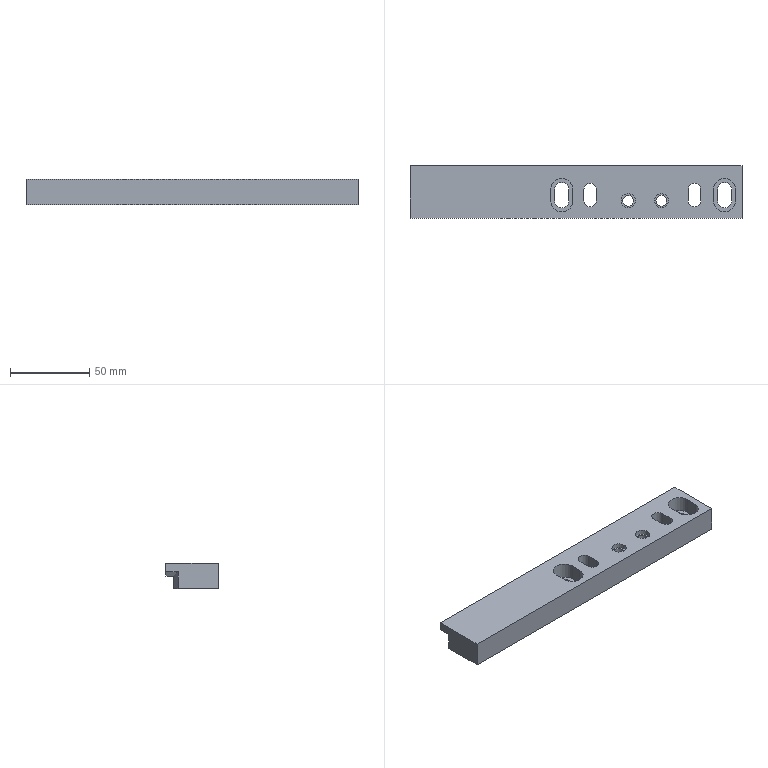Part | STEP file | lll_id4690_x_t | 1 solid | 44 faces | box 210 x 33 x 16 mm | volume 90799 mm3 | plane 28 | cylinder 16 | commonest cylinder face diameters 9 x6 8 x4 14 x4 6.8 x2
STEP:
#1=CARTESIAN_POINT('',(258.835,-359.7,13.));
#2=VERTEX_POINT('',#1);
#3=CARTESIAN_POINT('',(255.435,-359.7,13.));
#4=DIRECTION('',(0.,0.,-1.));
#5=DIRECTION('',(1.,0.,0.));
#6=AXIS2_PLACEMENT_3D('',#3,#4,#5);
#7=CIRCLE('',#6,3.4);
#8=EDGE_CURVE('',#2,#2,#7,.T.);
#9=ORIENTED_EDGE('',*,*,#8,.T.);
#10=EDGE_LOOP('',(#9));
#11=FACE_BOUND('',#10,.T.);
#12=CARTESIAN_POINT('',(250.935,-359.7,13.));
#13=VERTEX_POINT('',#12);
#14=CARTESIAN_POINT('',(255.435,-359.7,13.));
#15=DIRECTION('',(0.,0.,1.));
#16=DIRECTION('',(-1.,0.,0.));
#17=AXIS2_PLACEMENT_3D('',#14,#15,#16);
#18=CIRCLE('',#17,4.5);
#19=EDGE_CURVE('',#13,#13,#18,.T.);
#20=ORIENTED_EDGE('',*,*,#19,.T.);
#21=EDGE_LOOP('',(#20));
#22=FACE_BOUND('',#21,.T.);
#23=CARTESIAN_POINT('',(255.435,-359.7,13.));
#24=DIRECTION('',(0.,0.,-1.));
#25=DIRECTION('',(1.,0.,0.));
#26=AXIS2_PLACEMENT_3D('',#23,#24,#25);
#27=PLANE('',#26);
#28=ADVANCED_FACE('',(#11,#22),#27,.F.);
#29=CARTESIAN_POINT('',(311.935,-359.7,6.));
#30=VERTEX_POINT('',#29);
#31=CARTESIAN_POINT('',(311.935,-352.7,6.));
#32=VERTEX_POINT('',#31);
#33=CARTESIAN_POINT('',(311.935,-352.7,6.));
#34=DIRECTION('',(0.,1.,0.));
#35=VECTOR('',#34,1.);
#36=LINE('',#33,#35);
#37=EDGE_CURVE('',#30,#32,#36,.T.);
#38=ORIENTED_EDGE('',*,*,#37,.T.);
#39=CARTESIAN_POINT('',(320.935,-352.7,6.));
#40=VERTEX_POINT('',#39);
#41=CARTESIAN_POINT('',(316.435,-352.7,6.));
#42=DIRECTION('',(0.,0.,-1.));
#43=DIRECTION('',(1.,0.,0.));
#44=AXIS2_PLACEMENT_3D('',#41,#42,#43);
#45=CIRCLE('',#44,4.5);
#46=EDGE_CURVE('',#32,#40,#45,.T.);
#47=ORIENTED_EDGE('',*,*,#46,.T.);
#48=CARTESIAN_POINT('',(320.935,-359.7,6.));
#49=VERTEX_POINT('',#48);
#50=CARTESIAN_POINT('',(320.935,-359.7,6.));
#51=DIRECTION('',(0.,-1.,0.));
#52=VECTOR('',#51,1.);
#53=LINE('',#50,#52);
#54=EDGE_CURVE('',#40,#49,#53,.T.);
#55=ORIENTED_EDGE('',*,*,#54,.T.);
#56=CARTESIAN_POINT('',(316.435,-359.7,6.));
#57=DIRECTION('',(0.,0.,-1.));
#58=DIRECTION('',(1.,0.,0.));
#59=AXIS2_PLACEMENT_3D('',#56,#57,#58);
#60=CIRCLE('',#59,4.5);
#61=EDGE_CURVE('',#49,#30,#60,.T.);
#62=ORIENTED_EDGE('',*,*,#61,.T.);
#63=EDGE_LOOP('',(#38,#47,#55,#62));
#64=FACE_BOUND('',#63,.T.);
#65=CARTESIAN_POINT('',(323.435,-352.7,6.));
#66=VERTEX_POINT('',#65);
#67=CARTESIAN_POINT('',(309.435,-352.7,6.));
#68=VERTEX_POINT('',#67);
#69=CARTESIAN_POINT('',(316.435,-352.7,6.));
#70=DIRECTION('',(0.,0.,1.));
#71=DIRECTION('',(-1.,0.,0.));
#72=AXIS2_PLACEMENT_3D('',#69,#70,#71);
#73=CIRCLE('',#72,7.);
#74=EDGE_CURVE('',#66,#68,#73,.T.);
#75=ORIENTED_EDGE('',*,*,#74,.T.);
#76=CARTESIAN_POINT('',(309.435,-359.7,6.));
#77=VERTEX_POINT('',#76);
#78=CARTESIAN_POINT('',(309.435,-359.7,6.));
#79=DIRECTION('',(0.,-1.,0.));
#80=VECTOR('',#79,1.);
#81=LINE('',#78,#80);
#82=EDGE_CURVE('',#68,#77,#81,.T.);
#83=ORIENTED_EDGE('',*,*,#82,.T.);
#84=CARTESIAN_POINT('',(323.435,-359.7,6.));
#85=VERTEX_POINT('',#84);
#86=CARTESIAN_POINT('',(316.435,-359.7,6.));
#87=DIRECTION('',(0.,0.,1.));
#88=DIRECTION('',(-1.,0.,0.));
#89=AXIS2_PLACEMENT_3D('',#86,#87,#88);
#90=CIRCLE('',#89,7.);
#91=EDGE_CURVE('',#77,#85,#90,.T.);
#92=ORIENTED_EDGE('',*,*,#91,.T.);
#93=CARTESIAN_POINT('',(323.435,-352.7,6.));
#94=DIRECTION('',(0.,1.,0.));
#95=VECTOR('',#94,1.);
#96=LINE('',#93,#95);
#97=EDGE_CURVE('',#85,#66,#96,.T.);
#98=ORIENTED_EDGE('',*,*,#97,.T.);
#99=EDGE_LOOP('',(#75,#83,#92,#98));
#100=FACE_BOUND('',#99,.T.);
#101=CARTESIAN_POINT('',(316.435,-352.7,6.));
#102=DIRECTION('',(0.,0.,-1.));
#103=DIRECTION('',(1.,0.,0.));
#104=AXIS2_PLACEMENT_3D('',#101,#102,#103);
#105=PLANE('',#104);
#106=ADVANCED_FACE('',(#64,#100),#105,.F.);
#107=CARTESIAN_POINT('',(206.435,-359.7,6.));
#108=VERTEX_POINT('',#107);
#109=CARTESIAN_POINT('',(220.435,-359.7,6.));
#110=VERTEX_POINT('',#109);
#111=CARTESIAN_POINT('',(213.435,-359.7,6.));
#112=DIRECTION('',(0.,0.,1.));
#113=DIRECTION('',(-1.,0.,0.));
#114=AXIS2_PLACEMENT_3D('',#111,#112,#113);
#115=CIRCLE('',#114,7.);
#116=EDGE_CURVE('',#108,#110,#115,.T.);
#117=ORIENTED_EDGE('',*,*,#116,.T.);
#118=CARTESIAN_POINT('',(220.435,-352.7,6.));
#119=VERTEX_POINT('',#118);
#120=CARTESIAN_POINT('',(220.435,-352.7,6.));
#121=DIRECTION('',(0.,1.,0.));
#122=VECTOR('',#121,1.);
#123=LINE('',#120,#122);
#124=EDGE_CURVE('',#110,#119,#123,.T.);
#125=ORIENTED_EDGE('',*,*,#124,.T.);
#126=CARTESIAN_POINT('',(206.435,-352.7,6.));
#127=VERTEX_POINT('',#126);
#128=CARTESIAN_POINT('',(213.435,-352.7,6.));
#129=DIRECTION('',(0.,0.,1.));
#130=DIRECTION('',(-1.,0.,0.));
#131=AXIS2_PLACEMENT_3D('',#128,#129,#130);
#132=CIRCLE('',#131,7.);
#133=EDGE_CURVE('',#119,#127,#132,.T.);
#134=ORIENTED_EDGE('',*,*,#133,.T.);
#135=CARTESIAN_POINT('',(206.435,-359.7,6.));
#136=DIRECTION('',(0.,-1.,0.));
#137=VECTOR('',#136,1.);
#138=LINE('',#135,#137);
#139=EDGE_CURVE('',#127,#108,#138,.T.);
#140=ORIENTED_EDGE('',*,*,#139,.T.);
#141=EDGE_LOOP('',(#117,#125,#134,#140));
#142=FACE_BOUND('',#141,.T.);
#143=CARTESIAN_POINT('',(217.935,-359.7,6.));
#144=VERTEX_POINT('',#143);
#145=CARTESIAN_POINT('',(217.935,-352.7,6.));
#146=VERTEX_POINT('',#145);
#147=CARTESIAN_POINT('',(217.935,-352.7,6.));
#148=DIRECTION('',(0.,1.,0.));
#149=VECTOR('',#148,1.);
#150=LINE('',#147,#149);
#151=EDGE_CURVE('',#144,#146,#150,.T.);
#152=ORIENTED_EDGE('',*,*,#151,.F.);
#153=CARTESIAN_POINT('',(208.935,-359.7,6.));
#154=VERTEX_POINT('',#153);
#155=CARTESIAN_POINT('',(213.435,-359.7,6.));
#156=DIRECTION('',(0.,0.,1.));
#157=DIRECTION('',(1.,0.,0.));
#158=AXIS2_PLACEMENT_3D('',#155,#156,#157);
#159=CIRCLE('',#158,4.5);
#160=EDGE_CURVE('',#154,#144,#159,.T.);
#161=ORIENTED_EDGE('',*,*,#160,.F.);
#162=CARTESIAN_POINT('',(208.935,-352.7,6.));
#163=VERTEX_POINT('',#162);
#164=CARTESIAN_POINT('',(208.935,-359.7,6.));
#165=DIRECTION('',(0.,-1.,0.));
#166=VECTOR('',#165,1.);
#167=LINE('',#164,#166);
#168=EDGE_CURVE('',#163,#154,#167,.T.);
#169=ORIENTED_EDGE('',*,*,#168,.F.);
#170=CARTESIAN_POINT('',(213.435,-352.7,6.));
#171=DIRECTION('',(0.,0.,1.));
#172=DIRECTION('',(1.,0.,0.));
#173=AXIS2_PLACEMENT_3D('',#170,#171,#172);
#174=CIRCLE('',#173,4.5);
#175=EDGE_CURVE('',#146,#163,#174,.T.);
#176=ORIENTED_EDGE('',*,*,#175,.F.);
#177=EDGE_LOOP('',(#152,#161,#169,#176));
#178=FACE_BOUND('',#177,.T.);
#179=CARTESIAN_POINT('',(213.435,-359.7,6.));
#180=DIRECTION('',(0.,0.,-1.));
#181=DIRECTION('',(1.,0.,0.));
#182=AXIS2_PLACEMENT_3D('',#179,#180,#181);
#183=PLANE('',#182);
#184=ADVANCED_FACE('',(#142,#178),#183,.F.);
#185=CARTESIAN_POINT('',(117.435,-345.379,10.679));
#186=VERTEX_POINT('',#185);
#187=CARTESIAN_POINT('',(127.434,-342.7,8.));
#188=VERTEX_POINT('',#187);
#189=CARTESIAN_POINT('',(127.434,-342.7,8.));
#190=DIRECTION('',(0.9351,0.2506,-0.2506));
#191=VECTOR('',#190,1.);
#192=LINE('',#189,#191);
#193=EDGE_CURVE('',#186,#188,#192,.T.);
#194=ORIENTED_EDGE('',*,*,#193,.F.);
#195=CARTESIAN_POINT('',(117.435,-337.7,10.679));
#196=VERTEX_POINT('',#195);
#197=CARTESIAN_POINT('',(117.435,-345.379,10.679));
#198=DIRECTION('',(0.,-1.,0.));
#199=VECTOR('',#198,1.);
#200=LINE('',#197,#199);
#201=EDGE_CURVE('',#196,#186,#200,.T.);
#202=ORIENTED_EDGE('',*,*,#201,.F.);
#203=CARTESIAN_POINT('',(127.435,-337.7,8.));
#204=VERTEX_POINT('',#203);
#205=CARTESIAN_POINT('',(127.435,-337.7,8.));
#206=DIRECTION('',(-0.9659,0.,0.2588));
#207=VECTOR('',#206,1.);
#208=LINE('',#205,#207);
#209=EDGE_CURVE('',#204,#196,#208,.T.);
#210=ORIENTED_EDGE('',*,*,#209,.F.);
#211=CARTESIAN_POINT('',(127.435,-342.7,8.));
#212=VERTEX_POINT('',#211);
#213=CARTESIAN_POINT('',(127.435,-337.7,8.));
#214=DIRECTION('',(0.,1.,0.));
#215=VECTOR('',#214,1.);
#216=LINE('',#213,#215);
#217=EDGE_CURVE('',#212,#204,#216,.T.);
#218=ORIENTED_EDGE('',*,*,#217,.F.);
#219=CARTESIAN_POINT('',(183.414,-342.7,-7.));
#220=DIRECTION('',(0.9659,0.,-0.2588));
#221=VECTOR('',#220,1.);
#222=LINE('',#219,#221);
#223=EDGE_CURVE('',#188,#212,#222,.T.);
#224=ORIENTED_EDGE('',*,*,#223,.F.);
#225=EDGE_LOOP('',(#194,#202,#210,#218,#224));
#226=FACE_OUTER_BOUND('',#225,.T.);
#227=CARTESIAN_POINT('',(127.435,-317.091,8.));
#228=DIRECTION('',(-0.2588,0.,-0.9659));
#229=DIRECTION('',(0.9659,0.,-0.2588));
#230=AXIS2_PLACEMENT_3D('',#227,#228,#229);
#231=PLANE('',#230);
#232=ADVANCED_FACE('',(#226),#231,.T.);
#233=CARTESIAN_POINT('',(317.435,-337.7,8.));
#234=VERTEX_POINT('',#233);
#235=CARTESIAN_POINT('',(227.435,-337.7,8.));
#236=DIRECTION('',(1.,0.,0.));
#237=VECTOR('',#236,1.);
#238=LINE('',#235,#237);
#239=EDGE_CURVE('',#204,#234,#238,.T.);
#240=ORIENTED_EDGE('',*,*,#239,.T.);
#241=CARTESIAN_POINT('',(317.435,-342.701,8.));
#242=VERTEX_POINT('',#241);
#243=CARTESIAN_POINT('',(317.435,-345.38,8.));
#244=DIRECTION('',(0.,-1.,0.));
#245=VECTOR('',#244,1.);
#246=LINE('',#243,#245);
#247=EDGE_CURVE('',#234,#242,#246,.T.);
#248=ORIENTED_EDGE('',*,*,#247,.T.);
#249=CARTESIAN_POINT('',(317.434,-342.7,8.));
#250=VERTEX_POINT('',#249);
#251=CARTESIAN_POINT('',(327.435,-345.38,8.));
#252=DIRECTION('',(0.9659,-0.2588,0.));
#253=VECTOR('',#252,1.);
#254=LINE('',#251,#253);
#255=EDGE_CURVE('',#250,#242,#254,.T.);
#256=ORIENTED_EDGE('',*,*,#255,.F.);
#257=CARTESIAN_POINT('',(217.434,-342.7,8.));
#258=DIRECTION('',(1.,0.,0.));
#259=VECTOR('',#258,1.);
#260=LINE('',#257,#259);
#261=EDGE_CURVE('',#212,#250,#260,.T.);
#262=ORIENTED_EDGE('',*,*,#261,.F.);
#263=ORIENTED_EDGE('',*,*,#217,.T.);
#264=EDGE_LOOP('',(#240,#248,#256,#262,#263));
#265=FACE_OUTER_BOUND('',#264,.T.);
#266=CARTESIAN_POINT('',(249.706,-317.091,8.));
#267=DIRECTION('',(0.,0.,-1.));
#268=DIRECTION('',(1.,0.,0.));
#269=AXIS2_PLACEMENT_3D('',#266,#267,#268);
#270=PLANE('',#269);
#271=ADVANCED_FACE('',(#265),#270,.T.);
#272=CARTESIAN_POINT('',(327.435,-337.7,10.679));
#273=VERTEX_POINT('',#272);
#274=CARTESIAN_POINT('',(317.435,-337.7,8.));
#275=DIRECTION('',(-0.9659,0.,-0.2588));
#276=VECTOR('',#275,1.);
#277=LINE('',#274,#276);
#278=EDGE_CURVE('',#273,#234,#277,.T.);
#279=ORIENTED_EDGE('',*,*,#278,.F.);
#280=CARTESIAN_POINT('',(327.435,-345.38,10.679));
#281=VERTEX_POINT('',#280);
#282=CARTESIAN_POINT('',(327.435,-337.7,10.679));
#283=DIRECTION('',(0.,1.,0.));
#284=VECTOR('',#283,1.);
#285=LINE('',#282,#284);
#286=EDGE_CURVE('',#281,#273,#285,.T.);
#287=ORIENTED_EDGE('',*,*,#286,.F.);
#288=CARTESIAN_POINT('',(326.807,-345.212,10.511));
#289=DIRECTION('',(0.9351,-0.2506,0.2506));
#290=VECTOR('',#289,1.);
#291=LINE('',#288,#290);
#292=EDGE_CURVE('',#242,#281,#291,.T.);
#293=ORIENTED_EDGE('',*,*,#292,.F.);
#294=ORIENTED_EDGE('',*,*,#247,.F.);
#295=EDGE_LOOP('',(#279,#287,#293,#294));
#296=FACE_OUTER_BOUND('',#295,.T.);
#297=CARTESIAN_POINT('',(317.435,-317.091,8.));
#298=DIRECTION('',(0.2588,0.,-0.9659));
#299=DIRECTION('',(0.9659,0.,0.2588));
#300=AXIS2_PLACEMENT_3D('',#297,#298,#299);
#301=PLANE('',#300);
#302=ADVANCED_FACE('',(#296),#301,.T.);
#303=ORIENTED_EDGE('',*,*,#8,.F.);
#304=EDGE_LOOP('',(#303));
#305=FACE_BOUND('',#304,.T.);
#306=CARTESIAN_POINT('',(252.035,-359.7,0.));
#307=VERTEX_POINT('',#306);
#308=CARTESIAN_POINT('',(255.435,-359.7,0.));
#309=DIRECTION('',(0.,0.,1.));
#310=DIRECTION('',(-1.,0.,0.));
#311=AXIS2_PLACEMENT_3D('',#308,#309,#310);
#312=CIRCLE('',#311,3.4);
#313=EDGE_CURVE('',#307,#307,#312,.T.);
#314=ORIENTED_EDGE('',*,*,#313,.F.);
#315=EDGE_LOOP('',(#314));
#316=FACE_BOUND('',#315,.T.);
#317=CARTESIAN_POINT('',(255.435,-359.7,47.));
#318=DIRECTION('',(0.,0.,-1.));
#319=DIRECTION('',(1.,0.,0.));
#320=AXIS2_PLACEMENT_3D('',#317,#318,#319);
#321=CYLINDRICAL_SURFACE('',#320,3.4);
#322=ADVANCED_FACE('',(#305,#316),#321,.F.);
#323=CARTESIAN_POINT('',(317.434,-342.7,0.));
#324=VERTEX_POINT('',#323);
#325=CARTESIAN_POINT('',(127.434,-342.7,0.));
#326=VERTEX_POINT('',#325);
#327=CARTESIAN_POINT('',(217.434,-342.7,0.));
#328=DIRECTION('',(-1.,0.,0.));
#329=VECTOR('',#328,1.);
#330=LINE('',#327,#329);
#331=EDGE_CURVE('',#324,#326,#330,.T.);
#332=ORIENTED_EDGE('',*,*,#331,.T.);
#333=CARTESIAN_POINT('',(127.434,-342.7,8.));
#334=DIRECTION('',(0.,0.,1.));
#335=VECTOR('',#334,1.);
#336=LINE('',#333,#335);
#337=EDGE_CURVE('',#326,#188,#336,.T.);
#338=ORIENTED_EDGE('',*,*,#337,.T.);
#339=ORIENTED_EDGE('',*,*,#223,.T.);
#340=ORIENTED_EDGE('',*,*,#261,.T.);
#341=CARTESIAN_POINT('',(317.434,-342.7,8.));
#342=DIRECTION('',(0.,0.,1.));
#343=VECTOR('',#342,1.);
#344=LINE('',#341,#343);
#345=EDGE_CURVE('',#324,#250,#344,.T.);
#346=ORIENTED_EDGE('',*,*,#345,.F.);
#347=EDGE_LOOP('',(#332,#338,#339,#340,#346));
#348=FACE_OUTER_BOUND('',#347,.T.);
#349=CARTESIAN_POINT('',(217.434,-342.7,8.));
#350=DIRECTION('',(0.,-1.,0.));
#351=DIRECTION('',(0.,0.,1.));
#352=AXIS2_PLACEMENT_3D('',#349,#350,#351);
#353=PLANE('',#352);
#354=ADVANCED_FACE('',(#348),#353,.F.);
#355=CARTESIAN_POINT('',(117.435,-345.379,0.));
#356=VERTEX_POINT('',#355);
#357=CARTESIAN_POINT('',(127.434,-342.7,0.));
#358=DIRECTION('',(-0.9659,-0.2588,0.));
#359=VECTOR('',#358,1.);
#360=LINE('',#357,#359);
#361=EDGE_CURVE('',#326,#356,#360,.T.);
#362=ORIENTED_EDGE('',*,*,#361,.T.);
#363=CARTESIAN_POINT('',(117.435,-345.379,8.));
#364=DIRECTION('',(0.,0.,-1.));
#365=VECTOR('',#364,1.);
#366=LINE('',#363,#365);
#367=EDGE_CURVE('',#186,#356,#366,.T.);
#368=ORIENTED_EDGE('',*,*,#367,.F.);
#369=ORIENTED_EDGE('',*,*,#193,.T.);
#370=ORIENTED_EDGE('',*,*,#337,.F.);
#371=EDGE_LOOP('',(#362,#368,#369,#370));
#372=FACE_OUTER_BOUND('',#371,.T.);
#373=CARTESIAN_POINT('',(127.434,-342.7,8.));
#374=DIRECTION('',(0.2588,-0.9659,0.));
#375=DIRECTION('',(0.9659,0.2588,0.));
#376=AXIS2_PLACEMENT_3D('',#373,#374,#375);
#377=PLANE('',#376);
#378=ADVANCED_FACE('',(#372),#377,.F.);
#379=CARTESIAN_POINT('',(250.935,-359.7,16.));
#380=VERTEX_POINT('',#379);
#381=CARTESIAN_POINT('',(255.435,-359.7,16.));
#382=DIRECTION('',(0.,0.,1.));
#383=DIRECTION('',(-1.,0.,0.));
#384=AXIS2_PLACEMENT_3D('',#381,#382,#383);
#385=CIRCLE('',#384,4.5);
#386=EDGE_CURVE('',#380,#380,#385,.T.);
#387=ORIENTED_EDGE('',*,*,#386,.T.);
#388=EDGE_LOOP('',(#387));
#389=FACE_BOUND('',#388,.T.);
#390=ORIENTED_EDGE('',*,*,#19,.F.);
#391=EDGE_LOOP('',(#390));
#392=FACE_BOUND('',#391,.T.);
#393=CARTESIAN_POINT('',(255.435,-359.7,47.));
#394=DIRECTION('',(0.,0.,-1.));
#395=DIRECTION('',(1.,0.,0.));
#396=AXIS2_PLACEMENT_3D('',#393,#394,#395);
#397=CYLINDRICAL_SURFACE('',#396,4.5);
#398=ADVANCED_FACE('',(#389,#392),#397,.F.);
#399=CARTESIAN_POINT('',(309.435,-352.7,16.));
#400=VERTEX_POINT('',#399);
#401=CARTESIAN_POINT('',(309.435,-359.7,16.));
#402=VERTEX_POINT('',#401);
#403=CARTESIAN_POINT('',(309.435,-370.7,16.));
#404=DIRECTION('',(0.,-1.,0.));
#405=VECTOR('',#404,1.);
#406=LINE('',#403,#405);
#407=EDGE_CURVE('',#400,#402,#406,.T.);
#408=ORIENTED_EDGE('',*,*,#407,.T.);
#409=CARTESIAN_POINT('',(309.435,-359.7,47.));
#410=DIRECTION('',(0.,0.,1.));
#411=VECTOR('',#410,1.);
#412=LINE('',#409,#411);
#413=EDGE_CURVE('',#77,#402,#412,.T.);
#414=ORIENTED_EDGE('',*,*,#413,.F.);
#415=ORIENTED_EDGE('',*,*,#82,.F.);
#416=CARTESIAN_POINT('',(309.435,-352.7,47.));
#417=DIRECTION('',(0.,0.,1.));
#418=VECTOR('',#417,1.);
#419=LINE('',#416,#418);
#420=EDGE_CURVE('',#68,#400,#419,.T.);
#421=ORIENTED_EDGE('',*,*,#420,.T.);
#422=EDGE_LOOP('',(#408,#414,#415,#421));
#423=FACE_OUTER_BOUND('',#422,.T.);
#424=CARTESIAN_POINT('',(309.435,-359.7,47.));
#425=DIRECTION('',(-1.,0.,0.));
#426=DIRECTION('',(0.,0.,-1.));
#427=AXIS2_PLACEMENT_3D('',#424,#425,#426);
#428=PLANE('',#427);
#429=ADVANCED_FACE('',(#423),#428,.F.);
#430=CARTESIAN_POINT('',(323.435,-359.7,16.));
#431=VERTEX_POINT('',#430);
#432=CARTESIAN_POINT('',(316.435,-359.7,16.));
#433=DIRECTION('',(0.,0.,1.));
#434=DIRECTION('',(-1.,0.,0.));
#435=AXIS2_PLACEMENT_3D('',#432,#433,#434);
#436=CIRCLE('',#435,7.);
#437=EDGE_CURVE('',#402,#431,#436,.T.);
#438=ORIENTED_EDGE('',*,*,#437,.T.);
#439=CARTESIAN_POINT('',(323.435,-359.7,47.));
#440=DIRECTION('',(0.,0.,1.));
#441=VECTOR('',#440,1.);
#442=LINE('',#439,#441);
#443=EDGE_CURVE('',#85,#431,#442,.T.);
#444=ORIENTED_EDGE('',*,*,#443,.F.);
#445=ORIENTED_EDGE('',*,*,#91,.F.);
#446=ORIENTED_EDGE('',*,*,#413,.T.);
#447=EDGE_LOOP('',(#438,#444,#445,#446));
#448=FACE_OUTER_BOUND('',#447,.T.);
#449=CARTESIAN_POINT('',(316.435,-359.7,47.));
#450=DIRECTION('',(0.,0.,-1.));
#451=DIRECTION('',(1.,0.,0.));
#452=AXIS2_PLACEMENT_3D('',#449,#450,#451);
#453=CYLINDRICAL_SURFACE('',#452,7.);
#454=ADVANCED_FACE('',(#448),#453,.F.);
#455=CARTESIAN_POINT('',(323.435,-352.7,16.));
#456=VERTEX_POINT('',#455);
#457=CARTESIAN_POINT('',(323.435,-370.7,16.));
#458=DIRECTION('',(0.,1.,0.));
#459=VECTOR('',#458,1.);
#460=LINE('',#457,#459);
#461=EDGE_CURVE('',#431,#456,#460,.T.);
#462=ORIENTED_EDGE('',*,*,#461,.T.);
#463=CARTESIAN_POINT('',(323.435,-352.7,47.));
#464=DIRECTION('',(0.,0.,1.));
#465=VECTOR('',#464,1.);
#466=LINE('',#463,#465);
#467=EDGE_CURVE('',#66,#456,#466,.T.);
#468=ORIENTED_EDGE('',*,*,#467,.F.);
#469=ORIENTED_EDGE('',*,*,#97,.F.);
#470=ORIENTED_EDGE('',*,*,#443,.T.);
#471=EDGE_LOOP('',(#462,#468,#469,#470));
#472=FACE_OUTER_BOUND('',#471,.T.);
#473=CARTESIAN_POINT('',(323.435,-352.7,47.));
#474=DIRECTION('',(1.,0.,0.));
#475=DIRECTION('',(0.,0.,1.));
#476=AXIS2_PLACEMENT_3D('',#473,#474,#475);
#477=PLANE('',#476);
#478=ADVANCED_FACE('',(#472),#477,.F.);
#479=CARTESIAN_POINT('',(316.435,-352.7,16.));
#480=DIRECTION('',(0.,0.,1.));
#481=DIRECTION('',(-1.,0.,0.));
#482=AXIS2_PLACEMENT_3D('',#479,#480,#481);
#483=CIRCLE('',#482,7.);
#484=EDGE_CURVE('',#456,#400,#483,.T.);
#485=ORIENTED_EDGE('',*,*,#484,.T.);
#486=ORIENTED_EDGE('',*,*,#420,.F.);
#487=ORIENTED_EDGE('',*,*,#74,.F.);
#488=ORIENTED_EDGE('',*,*,#467,.T.);
#489=EDGE_LOOP('',(#485,#486,#487,#488));
#490=FACE_OUTER_BOUND('',#489,.T.);
#491=CARTESIAN_POINT('',(316.435,-352.7,47.));
#492=DIRECTION('',(0.,0.,-1.));
#493=DIRECTION('',(1.,0.,0.));
#494=AXIS2_PLACEMENT_3D('',#491,#492,#493);
#495=CYLINDRICAL_SURFACE('',#494,7.);
#496=ADVANCED_FACE('',(#490),#495,.F.);
#497=CARTESIAN_POINT('',(220.435,-359.7,16.));
#498=VERTEX_POINT('',#497);
#499=CARTESIAN_POINT('',(220.435,-352.7,16.));
#500=VERTEX_POINT('',#499);
#501=CARTESIAN_POINT('',(220.435,-370.7,16.));
#502=DIRECTION('',(0.,1.,0.));
#503=VECTOR('',#502,1.);
#504=LINE('',#501,#503);
#505=EDGE_CURVE('',#498,#500,#504,.T.);
#506=ORIENTED_EDGE('',*,*,#505,.T.);
#507=CARTESIAN_POINT('',(220.435,-352.7,47.));
#508=DIRECTION('',(0.,0.,1.));
#509=VECTOR('',#508,1.);
#510=LINE('',#507,#509);
#511=EDGE_CURVE('',#119,#500,#510,.T.);
#512=ORIENTED_EDGE('',*,*,#511,.F.);
#513=ORIENTED_EDGE('',*,*,#124,.F.);
#514=CARTESIAN_POINT('',(220.435,-359.7,47.));
#515=DIRECTION('',(0.,0.,1.));
#516=VECTOR('',#515,1.);
#517=LINE('',#514,#516);
#518=EDGE_CURVE('',#110,#498,#517,.T.);
#519=ORIENTED_EDGE('',*,*,#518,.T.);
#520=EDGE_LOOP('',(#506,#512,#513,#519));
#521=FACE_OUTER_BOUND('',#520,.T.);
#522=CARTESIAN_POINT('',(220.435,-352.7,47.));
#523=DIRECTION('',(1.,0.,0.));
#524=DIRECTION('',(0.,0.,1.));
#525=AXIS2_PLACEMENT_3D('',#522,#523,#524);
#526=PLANE('',#525);
#527=ADVANCED_FACE('',(#521),#526,.F.);
#528=CARTESIAN_POINT('',(206.435,-352.7,16.));
#529=VERTEX_POINT('',#528);
#530=CARTESIAN_POINT('',(213.435,-352.7,16.));
#531=DIRECTION('',(0.,0.,1.));
#532=DIRECTION('',(-1.,0.,0.));
#533=AXIS2_PLACEMENT_3D('',#530,#531,#532);
#534=CIRCLE('',#533,7.);
#535=EDGE_CURVE('',#500,#529,#534,.T.);
#536=ORIENTED_EDGE('',*,*,#535,.T.);
#537=CARTESIAN_POINT('',(206.435,-352.7,47.));
#538=DIRECTION('',(0.,0.,1.));
#539=VECTOR('',#538,1.);
#540=LINE('',#537,#539);
#541=EDGE_CURVE('',#127,#529,#540,.T.);
#542=ORIENTED_EDGE('',*,*,#541,.F.);
#543=ORIENTED_EDGE('',*,*,#133,.F.);
#544=ORIENTED_EDGE('',*,*,#511,.T.);
#545=EDGE_LOOP('',(#536,#542,#543,#544));
#546=FACE_OUTER_BOUND('',#545,.T.);
#547=CARTESIAN_POINT('',(213.435,-352.7,47.));
#548=DIRECTION('',(0.,0.,-1.));
#549=DIRECTION('',(1.,0.,0.));
#550=AXIS2_PLACEMENT_3D('',#547,#548,#549);
#551=CYLINDRICAL_SURFACE('',#550,7.);
#552=ADVANCED_FACE('',(#546),#551,.F.);
#553=CARTESIAN_POINT('',(206.435,-359.7,16.));
#554=VERTEX_POINT('',#553);
#555=CARTESIAN_POINT('',(206.435,-370.7,16.));
#556=DIRECTION('',(0.,-1.,0.));
#557=VECTOR('',#556,1.);
#558=LINE('',#555,#557);
#559=EDGE_CURVE('',#529,#554,#558,.T.);
#560=ORIENTED_EDGE('',*,*,#559,.T.);
#561=CARTESIAN_POINT('',(206.435,-359.7,47.));
#562=DIRECTION('',(0.,0.,1.));
#563=VECTOR('',#562,1.);
#564=LINE('',#561,#563);
#565=EDGE_CURVE('',#108,#554,#564,.T.);
#566=ORIENTED_EDGE('',*,*,#565,.F.);
#567=ORIENTED_EDGE('',*,*,#139,.F.);
#568=ORIENTED_EDGE('',*,*,#541,.T.);
#569=EDGE_LOOP('',(#560,#566,#567,#568));
#570=FACE_OUTER_BOUND('',#569,.T.);
#571=CARTESIAN_POINT('',(206.435,-359.7,47.));
#572=DIRECTION('',(-1.,0.,0.));
#573=DIRECTION('',(0.,0.,-1.));
#574=AXIS2_PLACEMENT_3D('',#571,#572,#573);
#575=PLANE('',#574);
#576=ADVANCED_FACE('',(#570),#575,.F.);
#577=CARTESIAN_POINT('',(213.435,-359.7,16.));
#578=DIRECTION('',(0.,0.,1.));
#579=DIRECTION('',(-1.,0.,0.));
#580=AXIS2_PLACEMENT_3D('',#577,#578,#579);
#581=CIRCLE('',#580,7.);
#582=EDGE_CURVE('',#554,#498,#581,.T.);
#583=ORIENTED_EDGE('',*,*,#582,.T.);
#584=ORIENTED_EDGE('',*,*,#518,.F.);
#585=ORIENTED_EDGE('',*,*,#116,.F.);
#586=ORIENTED_EDGE('',*,*,#565,.T.);
#587=EDGE_LOOP('',(#583,#584,#585,#586));
#588=FACE_OUTER_BOUND('',#587,.T.);
#589=CARTESIAN_POINT('',(213.435,-359.7,47.));
#590=DIRECTION('',(0.,0.,-1.));
#591=DIRECTION('',(1.,0.,0.));
#592=AXIS2_PLACEMENT_3D('',#589,#590,#591);
#593=CYLINDRICAL_SURFACE('',#592,7.);
#594=ADVANCED_FACE('',(#588),#593,.F.);
#595=CARTESIAN_POINT('',(117.435,-337.7,16.));
#596=VERTEX_POINT('',#595);
#597=CARTESIAN_POINT('',(117.435,-337.7,16.));
#598=DIRECTION('',(0.,0.,-1.));
#599=VECTOR('',#598,1.);
#600=LINE('',#597,#599);
#601=EDGE_CURVE('',#596,#196,#600,.T.);
#602=ORIENTED_EDGE('',*,*,#601,.T.);
#603=ORIENTED_EDGE('',*,*,#201,.T.);
#604=ORIENTED_EDGE('',*,*,#367,.T.);
#605=CARTESIAN_POINT('',(117.435,-370.7,0.));
#606=VERTEX_POINT('',#605);
#607=CARTESIAN_POINT('',(117.435,-337.7,0.));
#608=DIRECTION('',(0.,-1.,0.));
#609=VECTOR('',#608,1.);
#610=LINE('',#607,#609);
#611=EDGE_CURVE('',#356,#606,#610,.T.);
#612=ORIENTED_EDGE('',*,*,#611,.T.);
#613=CARTESIAN_POINT('',(117.435,-370.7,16.));
#614=VERTEX_POINT('',#613);
#615=CARTESIAN_POINT('',(117.435,-370.7,16.));
#616=DIRECTION('',(0.,0.,-1.));
#617=VECTOR('',#616,1.);
#618=LINE('',#615,#617);
#619=EDGE_CURVE('',#614,#606,#618,.T.);
#620=ORIENTED_EDGE('',*,*,#619,.F.);
#621=CARTESIAN_POINT('',(117.435,-337.7,16.));
#622=DIRECTION('',(0.,-1.,0.));
#623=VECTOR('',#622,1.);
#624=LINE('',#621,#623);
#625=EDGE_CURVE('',#596,#614,#624,.T.);
#626=ORIENTED_EDGE('',*,*,#625,.F.);
#627=EDGE_LOOP('',(#602,#603,#604,#612,#620,#626));
#628=FACE_OUTER_BOUND('',#627,.T.);
#629=CARTESIAN_POINT('',(117.435,-337.7,16.));
#630=DIRECTION('',(1.,0.,0.));
#631=DIRECTION('',(0.,0.,1.));
#632=AXIS2_PLACEMENT_3D('',#629,#630,#631);
#633=PLANE('',#632);
#634=ADVANCED_FACE('',(#628),#633,.F.);
#635=CARTESIAN_POINT('',(327.435,-337.7,16.));
#636=VERTEX_POINT('',#635);
#637=CARTESIAN_POINT('',(327.435,-337.7,16.));
#638=DIRECTION('',(0.,0.,-1.));
#639=VECTOR('',#638,1.);
#640=LINE('',#637,#639);
#641=EDGE_CURVE('',#636,#273,#640,.T.);
#642=ORIENTED_EDGE('',*,*,#641,.T.);
#643=ORIENTED_EDGE('',*,*,#278,.T.);
#644=ORIENTED_EDGE('',*,*,#239,.F.);
#645=ORIENTED_EDGE('',*,*,#209,.T.);
#646=ORIENTED_EDGE('',*,*,#601,.F.);
#647=CARTESIAN_POINT('',(227.435,-337.7,16.));
#648=DIRECTION('',(-1.,0.,0.));
#649=VECTOR('',#648,1.);
#650=LINE('',#647,#649);
#651=EDGE_CURVE('',#636,#596,#650,.T.);
#652=ORIENTED_EDGE('',*,*,#651,.F.);
#653=EDGE_LOOP('',(#642,#643,#644,#645,#646,#652));
#654=FACE_OUTER_BOUND('',#653,.T.);
#655=CARTESIAN_POINT('',(227.435,-337.7,16.));
#656=DIRECTION('',(0.,-1.,0.));
#657=DIRECTION('',(0.,0.,1.));
#658=AXIS2_PLACEMENT_3D('',#655,#656,#657);
#659=PLANE('',#658);
#660=ADVANCED_FACE('',(#654),#659,.F.);
#661=CARTESIAN_POINT('',(327.435,-345.38,0.));
#662=VERTEX_POINT('',#661);
#663=CARTESIAN_POINT('',(327.435,-345.38,8.));
#664=DIRECTION('',(0.,0.,-1.));
#665=VECTOR('',#664,1.);
#666=LINE('',#663,#665);
#667=EDGE_CURVE('',#281,#662,#666,.T.);
#668=ORIENTED_EDGE('',*,*,#667,.F.);
#669=ORIENTED_EDGE('',*,*,#286,.T.);
#670=ORIENTED_EDGE('',*,*,#641,.F.);
#671=CARTESIAN_POINT('',(327.435,-370.7,16.));
#672=VERTEX_POINT('',#671);
#673=CARTESIAN_POINT('',(327.435,-370.7,16.));
#674=DIRECTION('',(0.,1.,0.));
#675=VECTOR('',#674,1.);
#676=LINE('',#673,#675);
#677=EDGE_CURVE('',#672,#636,#676,.T.);
#678=ORIENTED_EDGE('',*,*,#677,.F.);
#679=CARTESIAN_POINT('',(327.435,-370.7,0.));
#680=VERTEX_POINT('',#679);
#681=CARTESIAN_POINT('',(327.435,-370.7,16.));
#682=DIRECTION('',(0.,0.,-1.));
#683=VECTOR('',#682,1.);
#684=LINE('',#681,#683);
#685=EDGE_CURVE('',#672,#680,#684,.T.);
#686=ORIENTED_EDGE('',*,*,#685,.T.);
#687=CARTESIAN_POINT('',(327.435,-370.7,0.));
#688=DIRECTION('',(0.,1.,0.));
#689=VECTOR('',#688,1.);
#690=LINE('',#687,#689);
#691=EDGE_CURVE('',#680,#662,#690,.T.);
#692=ORIENTED_EDGE('',*,*,#691,.T.);
#693=EDGE_LOOP('',(#668,#669,#670,#678,#686,#692));
#694=FACE_OUTER_BOUND('',#693,.T.);
#695=CARTESIAN_POINT('',(327.435,-370.7,16.));
#696=DIRECTION('',(-1.,0.,0.));
#697=DIRECTION('',(0.,0.,-1.));
#698=AXIS2_PLACEMENT_3D('',#695,#696,#697);
#699=PLANE('',#698);
#700=ADVANCED_FACE('',(#694),#699,.F.);
#701=CARTESIAN_POINT('',(147.435,-370.7,0.));
#702=DIRECTION('',(1.,0.,0.));
#703=VECTOR('',#702,1.);
#704=LINE('',#701,#703);
#705=EDGE_CURVE('',#606,#680,#704,.T.);
#706=ORIENTED_EDGE('',*,*,#705,.T.);
#707=ORIENTED_EDGE('',*,*,#685,.F.);
#708=CARTESIAN_POINT('',(147.435,-370.7,16.));
#709=DIRECTION('',(1.,0.,0.));
#710=VECTOR('',#709,1.);
#711=LINE('',#708,#710);
#712=EDGE_CURVE('',#614,#672,#711,.T.);
#713=ORIENTED_EDGE('',*,*,#712,.F.);
#714=ORIENTED_EDGE('',*,*,#619,.T.);
#715=EDGE_LOOP('',(#706,#707,#713,#714));
#716=FACE_OUTER_BOUND('',#715,.T.);
#717=CARTESIAN_POINT('',(147.435,-370.7,16.));
#718=DIRECTION('',(0.,1.,0.));
#719=DIRECTION('',(0.,0.,-1.));
#720=AXIS2_PLACEMENT_3D('',#717,#718,#719);
#721=PLANE('',#720);
#722=ADVANCED_FACE('',(#716),#721,.F.);
#723=CARTESIAN_POINT('',(235.435,-359.7,0.));
#724=VERTEX_POINT('',#723);
#725=CARTESIAN_POINT('',(235.435,-359.7,16.));
#726=VERTEX_POINT('',#725);
#727=CARTESIAN_POINT('',(235.435,-359.7,47.));
#728=DIRECTION('',(0.,0.,1.));
#729=VECTOR('',#728,1.);
#730=LINE('',#727,#729);
#731=EDGE_CURVE('',#724,#726,#730,.T.);
#732=ORIENTED_EDGE('',*,*,#731,.F.);
#733=CARTESIAN_POINT('',(227.435,-359.7,0.));
#734=VERTEX_POINT('',#733);
#735=CARTESIAN_POINT('',(231.435,-359.7,0.));
#736=DIRECTION('',(0.,0.,1.));
#737=DIRECTION('',(-1.,0.,0.));
#738=AXIS2_PLACEMENT_3D('',#735,#736,#737);
#739=CIRCLE('',#738,4.);
#740=EDGE_CURVE('',#734,#724,#739,.T.);
#741=ORIENTED_EDGE('',*,*,#740,.F.);
#742=CARTESIAN_POINT('',(227.435,-359.7,16.));
#743=VERTEX_POINT('',#742);
#744=CARTESIAN_POINT('',(227.435,-359.7,47.));
#745=DIRECTION('',(0.,0.,1.));
#746=VECTOR('',#745,1.);
#747=LINE('',#744,#746);
#748=EDGE_CURVE('',#734,#743,#747,.T.);
#749=ORIENTED_EDGE('',*,*,#748,.T.);
#750=CARTESIAN_POINT('',(231.435,-359.7,16.));
#751=DIRECTION('',(0.,0.,-1.));
#752=DIRECTION('',(-1.,0.,0.));
#753=AXIS2_PLACEMENT_3D('',#750,#751,#752);
#754=CIRCLE('',#753,4.);
#755=EDGE_CURVE('',#726,#743,#754,.T.);
#756=ORIENTED_EDGE('',*,*,#755,.F.);
#757=EDGE_LOOP('',(#732,#741,#749,#756));
#758=FACE_OUTER_BOUND('',#757,.T.);
#759=CARTESIAN_POINT('',(231.435,-359.7,47.));
#760=DIRECTION('',(0.,0.,-1.));
#761=DIRECTION('',(1.,0.,0.));
#762=AXIS2_PLACEMENT_3D('',#759,#760,#761);
#763=CYLINDRICAL_SURFACE('',#762,4.);
#764=ADVANCED_FACE('',(#758),#763,.F.);
#765=CARTESIAN_POINT('',(235.435,-352.7,0.));
#766=VERTEX_POINT('',#765);
#767=CARTESIAN_POINT('',(235.435,-352.7,16.));
#768=VERTEX_POINT('',#767);
#769=CARTESIAN_POINT('',(235.435,-352.7,47.));
#770=DIRECTION('',(0.,0.,1.));
#771=VECTOR('',#770,1.);
#772=LINE('',#769,#771);
#773=EDGE_CURVE('',#766,#768,#772,.T.);
#774=ORIENTED_EDGE('',*,*,#773,.F.);
#775=CARTESIAN_POINT('',(235.435,-359.7,0.));
#776=DIRECTION('',(0.,1.,0.));
#777=VECTOR('',#776,1.);
#778=LINE('',#775,#777);
#779=EDGE_CURVE('',#724,#766,#778,.T.);
#780=ORIENTED_EDGE('',*,*,#779,.F.);
#781=ORIENTED_EDGE('',*,*,#731,.T.);
#782=CARTESIAN_POINT('',(235.435,-370.7,16.));
#783=DIRECTION('',(0.,-1.,0.));
#784=VECTOR('',#783,1.);
#785=LINE('',#782,#784);
#786=EDGE_CURVE('',#768,#726,#785,.T.);
#787=ORIENTED_EDGE('',*,*,#786,.F.);
#788=EDGE_LOOP('',(#774,#780,#781,#787));
#789=FACE_OUTER_BOUND('',#788,.T.);
#790=CARTESIAN_POINT('',(235.435,-359.7,47.));
#791=DIRECTION('',(-1.,0.,0.));
#792=DIRECTION('',(0.,0.,-1.));
#793=AXIS2_PLACEMENT_3D('',#790,#791,#792);
#794=PLANE('',#793);
#795=ADVANCED_FACE('',(#789),#794,.T.);
#796=CARTESIAN_POINT('',(227.435,-352.7,0.));
#797=VERTEX_POINT('',#796);
#798=CARTESIAN_POINT('',(227.435,-352.7,16.));
#799=VERTEX_POINT('',#798);
#800=CARTESIAN_POINT('',(227.435,-352.7,47.));
#801=DIRECTION('',(0.,0.,1.));
#802=VECTOR('',#801,1.);
#803=LINE('',#800,#802);
#804=EDGE_CURVE('',#797,#799,#803,.T.);
#805=ORIENTED_EDGE('',*,*,#804,.F.);
#806=CARTESIAN_POINT('',(231.435,-352.7,0.));
#807=DIRECTION('',(0.,0.,1.));
#808=DIRECTION('',(-1.,0.,0.));
#809=AXIS2_PLACEMENT_3D('',#806,#807,#808);
#810=CIRCLE('',#809,4.);
#811=EDGE_CURVE('',#766,#797,#810,.T.);
#812=ORIENTED_EDGE('',*,*,#811,.F.);
#813=ORIENTED_EDGE('',*,*,#773,.T.);
#814=CARTESIAN_POINT('',(231.435,-352.7,16.));
#815=DIRECTION('',(0.,0.,-1.));
#816=DIRECTION('',(-1.,0.,0.));
#817=AXIS2_PLACEMENT_3D('',#814,#815,#816);
#818=CIRCLE('',#817,4.);
#819=EDGE_CURVE('',#799,#768,#818,.T.);
#820=ORIENTED_EDGE('',*,*,#819,.F.);
#821=EDGE_LOOP('',(#805,#812,#813,#820));
#822=FACE_OUTER_BOUND('',#821,.T.);
#823=CARTESIAN_POINT('',(231.435,-352.7,47.));
#824=DIRECTION('',(0.,0.,-1.));
#825=DIRECTION('',(1.,0.,0.));
#826=AXIS2_PLACEMENT_3D('',#823,#824,#825);
#827=CYLINDRICAL_SURFACE('',#826,4.);
#828=ADVANCED_FACE('',(#822),#827,.F.);
#829=ORIENTED_EDGE('',*,*,#748,.F.);
#830=CARTESIAN_POINT('',(227.435,-352.7,0.));
#831=DIRECTION('',(0.,-1.,0.));
#832=VECTOR('',#831,1.);
#833=LINE('',#830,#832);
#834=EDGE_CURVE('',#797,#734,#833,.T.);
#835=ORIENTED_EDGE('',*,*,#834,.F.);
#836=ORIENTED_EDGE('',*,*,#804,.T.);
#837=CARTESIAN_POINT('',(227.435,-370.7,16.));
#838=DIRECTION('',(0.,1.,0.));
#839=VECTOR('',#838,1.);
#840=LINE('',#837,#839);
#841=EDGE_CURVE('',#743,#799,#840,.T.);
#842=ORIENTED_EDGE('',*,*,#841,.F.);
#843=EDGE_LOOP('',(#829,#835,#836,#842));
#844=FACE_OUTER_BOUND('',#843,.T.);
#845=CARTESIAN_POINT('',(227.435,-352.7,47.));
#846=DIRECTION('',(1.,0.,0.));
#847=DIRECTION('',(0.,0.,1.));
#848=AXIS2_PLACEMENT_3D('',#845,#846,#847);
#849=PLANE('',#848);
#850=ADVANCED_FACE('',(#844),#849,.T.);
#851=CARTESIAN_POINT('',(301.435,-359.7,16.));
#852=VERTEX_POINT('',#851);
#853=CARTESIAN_POINT('',(301.435,-352.7,16.));
#854=VERTEX_POINT('',#853);
#855=CARTESIAN_POINT('',(301.435,-370.7,16.));
#856=DIRECTION('',(0.,1.,0.));
#857=VECTOR('',#856,1.);
#858=LINE('',#855,#857);
#859=EDGE_CURVE('',#852,#854,#858,.T.);
#860=ORIENTED_EDGE('',*,*,#859,.T.);
#861=CARTESIAN_POINT('',(301.435,-352.7,0.));
#862=VERTEX_POINT('',#861);
#863=CARTESIAN_POINT('',(301.435,-352.7,47.));
#864=DIRECTION('',(0.,0.,1.));
#865=VECTOR('',#864,1.);
#866=LINE('',#863,#865);
#867=EDGE_CURVE('',#862,#854,#866,.T.);
#868=ORIENTED_EDGE('',*,*,#867,.F.);
#869=CARTESIAN_POINT('',(301.435,-359.7,0.));
#870=VERTEX_POINT('',#869);
#871=CARTESIAN_POINT('',(301.435,-352.7,0.));
#872=DIRECTION('',(0.,-1.,0.));
#873=VECTOR('',#872,1.);
#874=LINE('',#871,#873);
#875=EDGE_CURVE('',#862,#870,#874,.T.);
#876=ORIENTED_EDGE('',*,*,#875,.T.);
#877=CARTESIAN_POINT('',(301.435,-359.7,47.));
#878=DIRECTION('',(0.,0.,1.));
#879=VECTOR('',#878,1.);
#880=LINE('',#877,#879);
#881=EDGE_CURVE('',#870,#852,#880,.T.);
#882=ORIENTED_EDGE('',*,*,#881,.T.);
#883=EDGE_LOOP('',(#860,#868,#876,#882));
#884=FACE_OUTER_BOUND('',#883,.T.);
#885=CARTESIAN_POINT('',(301.435,-352.7,47.));
#886=DIRECTION('',(1.,0.,0.));
#887=DIRECTION('',(0.,0.,1.));
#888=AXIS2_PLACEMENT_3D('',#885,#886,#887);
#889=PLANE('',#888);
#890=ADVANCED_FACE('',(#884),#889,.F.);
#891=CARTESIAN_POINT('',(293.435,-352.7,16.));
#892=VERTEX_POINT('',#891);
#893=CARTESIAN_POINT('',(297.435,-352.7,16.));
#894=DIRECTION('',(0.,0.,1.));
#895=DIRECTION('',(-1.,0.,0.));
#896=AXIS2_PLACEMENT_3D('',#893,#894,#895);
#897=CIRCLE('',#896,4.);
#898=EDGE_CURVE('',#854,#892,#897,.T.);
#899=ORIENTED_EDGE('',*,*,#898,.T.);
#900=CARTESIAN_POINT('',(293.435,-352.7,0.));
#901=VERTEX_POINT('',#900);
#902=CARTESIAN_POINT('',(293.435,-352.7,47.));
#903=DIRECTION('',(0.,0.,1.));
#904=VECTOR('',#903,1.);
#905=LINE('',#902,#904);
#906=EDGE_CURVE('',#901,#892,#905,.T.);
#907=ORIENTED_EDGE('',*,*,#906,.F.);
#908=CARTESIAN_POINT('',(297.435,-352.7,0.));
#909=DIRECTION('',(0.,0.,-1.));
#910=DIRECTION('',(-1.,0.,0.));
#911=AXIS2_PLACEMENT_3D('',#908,#909,#910);
#912=CIRCLE('',#911,4.);
#913=EDGE_CURVE('',#901,#862,#912,.T.);
#914=ORIENTED_EDGE('',*,*,#913,.T.);
#915=ORIENTED_EDGE('',*,*,#867,.T.);
#916=EDGE_LOOP('',(#899,#907,#914,#915));
#917=FACE_OUTER_BOUND('',#916,.T.);
#918=CARTESIAN_POINT('',(297.435,-352.7,47.));
#919=DIRECTION('',(0.,0.,-1.));
#920=DIRECTION('',(1.,0.,0.));
#921=AXIS2_PLACEMENT_3D('',#918,#919,#920);
#922=CYLINDRICAL_SURFACE('',#921,4.);
#923=ADVANCED_FACE('',(#917),#922,.F.);
#924=CARTESIAN_POINT('',(293.435,-359.7,16.));
#925=VERTEX_POINT('',#924);
#926=CARTESIAN_POINT('',(293.435,-370.7,16.));
#927=DIRECTION('',(0.,-1.,0.));
#928=VECTOR('',#927,1.);
#929=LINE('',#926,#928);
#930=EDGE_CURVE('',#892,#925,#929,.T.);
#931=ORIENTED_EDGE('',*,*,#930,.T.);
#932=CARTESIAN_POINT('',(293.435,-359.7,0.));
#933=VERTEX_POINT('',#932);
#934=CARTESIAN_POINT('',(293.435,-359.7,47.));
#935=DIRECTION('',(0.,0.,1.));
#936=VECTOR('',#935,1.);
#937=LINE('',#934,#936);
#938=EDGE_CURVE('',#933,#925,#937,.T.);
#939=ORIENTED_EDGE('',*,*,#938,.F.);
#940=CARTESIAN_POINT('',(293.435,-359.7,0.));
#941=DIRECTION('',(0.,1.,0.));
#942=VECTOR('',#941,1.);
#943=LINE('',#940,#942);
#944=EDGE_CURVE('',#933,#901,#943,.T.);
#945=ORIENTED_EDGE('',*,*,#944,.T.);
#946=ORIENTED_EDGE('',*,*,#906,.T.);
#947=EDGE_LOOP('',(#931,#939,#945,#946));
#948=FACE_OUTER_BOUND('',#947,.T.);
#949=CARTESIAN_POINT('',(293.435,-359.7,47.));
#950=DIRECTION('',(-1.,0.,0.));
#951=DIRECTION('',(0.,0.,-1.));
#952=AXIS2_PLACEMENT_3D('',#949,#950,#951);
#953=PLANE('',#952);
#954=ADVANCED_FACE('',(#948),#953,.F.);
#955=CARTESIAN_POINT('',(297.435,-359.7,16.));
#956=DIRECTION('',(0.,0.,1.));
#957=DIRECTION('',(-1.,0.,0.));
#958=AXIS2_PLACEMENT_3D('',#955,#956,#957);
#959=CIRCLE('',#958,4.);
#960=EDGE_CURVE('',#925,#852,#959,.T.);
#961=ORIENTED_EDGE('',*,*,#960,.T.);
#962=ORIENTED_EDGE('',*,*,#881,.F.);
#963=CARTESIAN_POINT('',(297.435,-359.7,0.));
#964=DIRECTION('',(0.,0.,-1.));
#965=DIRECTION('',(-1.,0.,0.));
#966=AXIS2_PLACEMENT_3D('',#963,#964,#965);
#967=CIRCLE('',#966,4.);
#968=EDGE_CURVE('',#870,#933,#967,.T.);
#969=ORIENTED_EDGE('',*,*,#968,.T.);
#970=ORIENTED_EDGE('',*,*,#938,.T.);
#971=EDGE_LOOP('',(#961,#962,#969,#970));
#972=FACE_OUTER_BOUND('',#971,.T.);
#973=CARTESIAN_POINT('',(297.435,-359.7,47.));
#974=DIRECTION('',(0.,0.,-1.));
#975=DIRECTION('',(1.,0.,0.));
#976=AXIS2_PLACEMENT_3D('',#973,#974,#975);
#977=CYLINDRICAL_SURFACE('',#976,4.);
#978=ADVANCED_FACE('',(#972),#977,.F.);
#979=CARTESIAN_POINT('',(280.935,-359.7,16.));
#980=VERTEX_POINT('',#979);
#981=CARTESIAN_POINT('',(276.435,-359.7,16.));
#982=DIRECTION('',(0.,0.,1.));
#983=DIRECTION('',(1.,0.,0.));
#984=AXIS2_PLACEMENT_3D('',#981,#982,#983);
#985=CIRCLE('',#984,4.5);
#986=EDGE_CURVE('',#980,#980,#985,.T.);
#987=ORIENTED_EDGE('',*,*,#986,.F.);
#988=EDGE_LOOP('',(#987));
#989=FACE_BOUND('',#988,.T.);
#990=ORIENTED_EDGE('',*,*,#960,.F.);
#991=ORIENTED_EDGE('',*,*,#930,.F.);
#992=ORIENTED_EDGE('',*,*,#898,.F.);
#993=ORIENTED_EDGE('',*,*,#859,.F.);
#994=EDGE_LOOP('',(#990,#991,#992,#993));
#995=FACE_BOUND('',#994,.T.);
#996=ORIENTED_EDGE('',*,*,#841,.T.);
#997=ORIENTED_EDGE('',*,*,#819,.T.);
#998=ORIENTED_EDGE('',*,*,#786,.T.);
#999=ORIENTED_EDGE('',*,*,#755,.T.);
#1000=EDGE_LOOP('',(#996,#997,#998,#999));
#1001=FACE_BOUND('',#1000,.T.);
#1002=ORIENTED_EDGE('',*,*,#712,.T.);
#1003=ORIENTED_EDGE('',*,*,#677,.T.);
#1004=ORIENTED_EDGE('',*,*,#651,.T.);
#1005=ORIENTED_EDGE('',*,*,#625,.T.);
#1006=EDGE_LOOP('',(#1002,#1003,#1004,#1005));
#1007=FACE_BOUND('',#1006,.T.);
#1008=ORIENTED_EDGE('',*,*,#582,.F.);
#1009=ORIENTED_EDGE('',*,*,#559,.F.);
#1010=ORIENTED_EDGE('',*,*,#535,.F.);
#1011=ORIENTED_EDGE('',*,*,#505,.F.);
#1012=EDGE_LOOP('',(#1008,#1009,#1010,#1011));
#1013=FACE_BOUND('',#1012,.T.);
#1014=ORIENTED_EDGE('',*,*,#484,.F.);
#1015=ORIENTED_EDGE('',*,*,#461,.F.);
#1016=ORIENTED_EDGE('',*,*,#437,.F.);
#1017=ORIENTED_EDGE('',*,*,#407,.F.);
#1018=EDGE_LOOP('',(#1014,#1015,#1016,#1017));
#1019=FACE_BOUND('',#1018,.T.);
#1020=ORIENTED_EDGE('',*,*,#386,.F.);
#1021=EDGE_LOOP('',(#1020));
#1022=FACE_BOUND('',#1021,.T.);
#1023=CARTESIAN_POINT('',(227.435,-370.7,16.));
#1024=DIRECTION('',(0.,0.,1.));
#1025=DIRECTION('',(-1.,0.,0.));
#1026=AXIS2_PLACEMENT_3D('',#1023,#1024,#1025);
#1027=PLANE('',#1026);
#1028=ADVANCED_FACE('',(#989,#995,#1001,#1007,#1013,#1019,#1022),#1027,.T.);
#1029=CARTESIAN_POINT('',(327.435,-345.38,0.));
#1030=DIRECTION('',(-0.9659,0.2588,0.));
#1031=VECTOR('',#1030,1.);
#1032=LINE('',#1029,#1031);
#1033=EDGE_CURVE('',#662,#324,#1032,.T.);
#1034=ORIENTED_EDGE('',*,*,#1033,.T.);
#1035=ORIENTED_EDGE('',*,*,#345,.T.);
#1036=ORIENTED_EDGE('',*,*,#255,.T.);
#1037=ORIENTED_EDGE('',*,*,#292,.T.);
#1038=ORIENTED_EDGE('',*,*,#667,.T.);
#1039=EDGE_LOOP('',(#1034,#1035,#1036,#1037,#1038));
#1040=FACE_OUTER_BOUND('',#1039,.T.);
#1041=CARTESIAN_POINT('',(327.435,-345.38,8.));
#1042=DIRECTION('',(-0.2588,-0.9659,0.));
#1043=DIRECTION('',(0.9659,-0.2588,0.));
#1044=AXIS2_PLACEMENT_3D('',#1041,#1042,#1043);
#1045=PLANE('',#1044);
#1046=ADVANCED_FACE('',(#1040),#1045,.F.);
#1047=ORIENTED_EDGE('',*,*,#46,.F.);
#1048=CARTESIAN_POINT('',(311.935,-352.7,0.));
#1049=VERTEX_POINT('',#1048);
#1050=CARTESIAN_POINT('',(311.935,-352.7,47.));
#1051=DIRECTION('',(0.,0.,1.));
#1052=VECTOR('',#1051,1.);
#1053=LINE('',#1050,#1052);
#1054=EDGE_CURVE('',#1049,#32,#1053,.T.);
#1055=ORIENTED_EDGE('',*,*,#1054,.F.);
#1056=CARTESIAN_POINT('',(320.935,-352.7,0.));
#1057=VERTEX_POINT('',#1056);
#1058=CARTESIAN_POINT('',(316.435,-352.7,0.));
#1059=DIRECTION('',(0.,0.,1.));
#1060=DIRECTION('',(-1.,0.,0.));
#1061=AXIS2_PLACEMENT_3D('',#1058,#1059,#1060);
#1062=CIRCLE('',#1061,4.5);
#1063=EDGE_CURVE('',#1057,#1049,#1062,.T.);
#1064=ORIENTED_EDGE('',*,*,#1063,.F.);
#1065=CARTESIAN_POINT('',(320.935,-352.7,47.));
#1066=DIRECTION('',(0.,0.,1.));
#1067=VECTOR('',#1066,1.);
#1068=LINE('',#1065,#1067);
#1069=EDGE_CURVE('',#1057,#40,#1068,.T.);
#1070=ORIENTED_EDGE('',*,*,#1069,.T.);
#1071=EDGE_LOOP('',(#1047,#1055,#1064,#1070));
#1072=FACE_OUTER_BOUND('',#1071,.T.);
#1073=CARTESIAN_POINT('',(316.435,-352.7,47.));
#1074=DIRECTION('',(0.,0.,-1.));
#1075=DIRECTION('',(1.,0.,0.));
#1076=AXIS2_PLACEMENT_3D('',#1073,#1074,#1075);
#1077=CYLINDRICAL_SURFACE('',#1076,4.5);
#1078=ADVANCED_FACE('',(#1072),#1077,.F.);
#1079=ORIENTED_EDGE('',*,*,#54,.F.);
#1080=ORIENTED_EDGE('',*,*,#1069,.F.);
#1081=CARTESIAN_POINT('',(320.935,-359.7,0.));
#1082=VERTEX_POINT('',#1081);
#1083=CARTESIAN_POINT('',(320.935,-359.7,0.));
#1084=DIRECTION('',(0.,1.,0.));
#1085=VECTOR('',#1084,1.);
#1086=LINE('',#1083,#1085);
#1087=EDGE_CURVE('',#1082,#1057,#1086,.T.);
#1088=ORIENTED_EDGE('',*,*,#1087,.F.);
#1089=CARTESIAN_POINT('',(320.935,-359.7,47.));
#1090=DIRECTION('',(0.,0.,1.));
#1091=VECTOR('',#1090,1.);
#1092=LINE('',#1089,#1091);
#1093=EDGE_CURVE('',#1082,#49,#1092,.T.);
#1094=ORIENTED_EDGE('',*,*,#1093,.T.);
#1095=EDGE_LOOP('',(#1079,#1080,#1088,#1094));
#1096=FACE_OUTER_BOUND('',#1095,.T.);
#1097=CARTESIAN_POINT('',(320.935,-359.7,47.));
#1098=DIRECTION('',(-1.,0.,0.));
#1099=DIRECTION('',(0.,0.,-1.));
#1100=AXIS2_PLACEMENT_3D('',#1097,#1098,#1099);
#1101=PLANE('',#1100);
#1102=ADVANCED_FACE('',(#1096),#1101,.T.);
#1103=ORIENTED_EDGE('',*,*,#61,.F.);
#1104=ORIENTED_EDGE('',*,*,#1093,.F.);
#1105=CARTESIAN_POINT('',(311.935,-359.7,0.));
#1106=VERTEX_POINT('',#1105);
#1107=CARTESIAN_POINT('',(316.435,-359.7,0.));
#1108=DIRECTION('',(0.,0.,1.));
#1109=DIRECTION('',(-1.,0.,0.));
#1110=AXIS2_PLACEMENT_3D('',#1107,#1108,#1109);
#1111=CIRCLE('',#1110,4.5);
#1112=EDGE_CURVE('',#1106,#1082,#1111,.T.);
#1113=ORIENTED_EDGE('',*,*,#1112,.F.);
#1114=CARTESIAN_POINT('',(311.935,-359.7,47.));
#1115=DIRECTION('',(0.,0.,1.));
#1116=VECTOR('',#1115,1.);
#1117=LINE('',#1114,#1116);
#1118=EDGE_CURVE('',#1106,#30,#1117,.T.);
#1119=ORIENTED_EDGE('',*,*,#1118,.T.);
#1120=EDGE_LOOP('',(#1103,#1104,#1113,#1119));
#1121=FACE_OUTER_BOUND('',#1120,.T.);
#1122=CARTESIAN_POINT('',(316.435,-359.7,47.));
#1123=DIRECTION('',(0.,0.,-1.));
#1124=DIRECTION('',(1.,0.,0.));
#1125=AXIS2_PLACEMENT_3D('',#1122,#1123,#1124);
#1126=CYLINDRICAL_SURFACE('',#1125,4.5);
#1127=ADVANCED_FACE('',(#1121),#1126,.F.);
#1128=ORIENTED_EDGE('',*,*,#37,.F.);
#1129=ORIENTED_EDGE('',*,*,#1118,.F.);
#1130=CARTESIAN_POINT('',(311.935,-352.7,0.));
#1131=DIRECTION('',(0.,-1.,0.));
#1132=VECTOR('',#1131,1.);
#1133=LINE('',#1130,#1132);
#1134=EDGE_CURVE('',#1049,#1106,#1133,.T.);
#1135=ORIENTED_EDGE('',*,*,#1134,.F.);
#1136=ORIENTED_EDGE('',*,*,#1054,.T.);
#1137=EDGE_LOOP('',(#1128,#1129,#1135,#1136));
#1138=FACE_OUTER_BOUND('',#1137,.T.);
#1139=CARTESIAN_POINT('',(311.935,-352.7,47.));
#1140=DIRECTION('',(1.,0.,0.));
#1141=DIRECTION('',(0.,0.,1.));
#1142=AXIS2_PLACEMENT_3D('',#1139,#1140,#1141);
#1143=PLANE('',#1142);
#1144=ADVANCED_FACE('',(#1138),#1143,.T.);
#1145=CARTESIAN_POINT('',(208.935,-359.7,0.));
#1146=VERTEX_POINT('',#1145);
#1147=CARTESIAN_POINT('',(208.935,-359.7,47.));
#1148=DIRECTION('',(0.,0.,1.));
#1149=VECTOR('',#1148,1.);
#1150=LINE('',#1147,#1149);
#1151=EDGE_CURVE('',#1146,#154,#1150,.T.);
#1152=ORIENTED_EDGE('',*,*,#1151,.T.);
#1153=ORIENTED_EDGE('',*,*,#160,.T.);
#1154=CARTESIAN_POINT('',(217.935,-359.7,0.));
#1155=VERTEX_POINT('',#1154);
#1156=CARTESIAN_POINT('',(217.935,-359.7,47.));
#1157=DIRECTION('',(0.,0.,1.));
#1158=VECTOR('',#1157,1.);
#1159=LINE('',#1156,#1158);
#1160=EDGE_CURVE('',#1155,#144,#1159,.T.);
#1161=ORIENTED_EDGE('',*,*,#1160,.F.);
#1162=CARTESIAN_POINT('',(213.435,-359.7,0.));
#1163=DIRECTION('',(0.,0.,-1.));
#1164=DIRECTION('',(-1.,0.,0.));
#1165=AXIS2_PLACEMENT_3D('',#1162,#1163,#1164);
#1166=CIRCLE('',#1165,4.5);
#1167=EDGE_CURVE('',#1155,#1146,#1166,.T.);
#1168=ORIENTED_EDGE('',*,*,#1167,.T.);
#1169=EDGE_LOOP('',(#1152,#1153,#1161,#1168));
#1170=FACE_OUTER_BOUND('',#1169,.T.);
#1171=CARTESIAN_POINT('',(213.435,-359.7,47.));
#1172=DIRECTION('',(0.,0.,-1.));
#1173=DIRECTION('',(1.,0.,0.));
#1174=AXIS2_PLACEMENT_3D('',#1171,#1172,#1173);
#1175=CYLINDRICAL_SURFACE('',#1174,4.5);
#1176=ADVANCED_FACE('',(#1170),#1175,.F.);
#1177=CARTESIAN_POINT('',(208.935,-352.7,0.));
#1178=VERTEX_POINT('',#1177);
#1179=CARTESIAN_POINT('',(208.935,-352.7,47.));
#1180=DIRECTION('',(0.,0.,1.));
#1181=VECTOR('',#1180,1.);
#1182=LINE('',#1179,#1181);
#1183=EDGE_CURVE('',#1178,#163,#1182,.T.);
#1184=ORIENTED_EDGE('',*,*,#1183,.T.);
#1185=ORIENTED_EDGE('',*,*,#168,.T.);
#1186=ORIENTED_EDGE('',*,*,#1151,.F.);
#1187=CARTESIAN_POINT('',(208.935,-359.7,0.));
#1188=DIRECTION('',(0.,1.,0.));
#1189=VECTOR('',#1188,1.);
#1190=LINE('',#1187,#1189);
#1191=EDGE_CURVE('',#1146,#1178,#1190,.T.);
#1192=ORIENTED_EDGE('',*,*,#1191,.T.);
#1193=EDGE_LOOP('',(#1184,#1185,#1186,#1192));
#1194=FACE_OUTER_BOUND('',#1193,.T.);
#1195=CARTESIAN_POINT('',(208.935,-359.7,47.));
#1196=DIRECTION('',(-1.,0.,0.));
#1197=DIRECTION('',(0.,0.,-1.));
#1198=AXIS2_PLACEMENT_3D('',#1195,#1196,#1197);
#1199=PLANE('',#1198);
#1200=ADVANCED_FACE('',(#1194),#1199,.F.);
#1201=CARTESIAN_POINT('',(217.935,-352.7,0.));
#1202=VERTEX_POINT('',#1201);
#1203=CARTESIAN_POINT('',(217.935,-352.7,47.));
#1204=DIRECTION('',(0.,0.,1.));
#1205=VECTOR('',#1204,1.);
#1206=LINE('',#1203,#1205);
#1207=EDGE_CURVE('',#1202,#146,#1206,.T.);
#1208=ORIENTED_EDGE('',*,*,#1207,.T.);
#1209=ORIENTED_EDGE('',*,*,#175,.T.);
#1210=ORIENTED_EDGE('',*,*,#1183,.F.);
#1211=CARTESIAN_POINT('',(213.435,-352.7,0.));
#1212=DIRECTION('',(0.,0.,-1.));
#1213=DIRECTION('',(-1.,0.,0.));
#1214=AXIS2_PLACEMENT_3D('',#1211,#1212,#1213);
#1215=CIRCLE('',#1214,4.5);
#1216=EDGE_CURVE('',#1178,#1202,#1215,.T.);
#1217=ORIENTED_EDGE('',*,*,#1216,.T.);
#1218=EDGE_LOOP('',(#1208,#1209,#1210,#1217));
#1219=FACE_OUTER_BOUND('',#1218,.T.);
#1220=CARTESIAN_POINT('',(213.435,-352.7,47.));
#1221=DIRECTION('',(0.,0.,-1.));
#1222=DIRECTION('',(1.,0.,0.));
#1223=AXIS2_PLACEMENT_3D('',#1220,#1221,#1222);
#1224=CYLINDRICAL_SURFACE('',#1223,4.5);
#1225=ADVANCED_FACE('',(#1219),#1224,.F.);
#1226=ORIENTED_EDGE('',*,*,#1160,.T.);
#1227=ORIENTED_EDGE('',*,*,#151,.T.);
#1228=ORIENTED_EDGE('',*,*,#1207,.F.);
#1229=CARTESIAN_POINT('',(217.935,-352.7,0.));
#1230=DIRECTION('',(0.,-1.,0.));
#1231=VECTOR('',#1230,1.);
#1232=LINE('',#1229,#1231);
#1233=EDGE_CURVE('',#1202,#1155,#1232,.T.);
#1234=ORIENTED_EDGE('',*,*,#1233,.T.);
#1235=EDGE_LOOP('',(#1226,#1227,#1228,#1234));
#1236=FACE_OUTER_BOUND('',#1235,.T.);
#1237=CARTESIAN_POINT('',(217.935,-352.7,47.));
#1238=DIRECTION('',(1.,0.,0.));
#1239=DIRECTION('',(0.,0.,1.));
#1240=AXIS2_PLACEMENT_3D('',#1237,#1238,#1239);
#1241=PLANE('',#1240);
#1242=ADVANCED_FACE('',(#1236),#1241,.F.);
#1243=ORIENTED_EDGE('',*,*,#1233,.F.);
#1244=ORIENTED_EDGE('',*,*,#1216,.F.);
#1245=ORIENTED_EDGE('',*,*,#1191,.F.);
#1246=ORIENTED_EDGE('',*,*,#1167,.F.);
#1247=EDGE_LOOP('',(#1243,#1244,#1245,#1246));
#1248=FACE_BOUND('',#1247,.T.);
#1249=ORIENTED_EDGE('',*,*,#1134,.T.);
#1250=ORIENTED_EDGE('',*,*,#1112,.T.);
#1251=ORIENTED_EDGE('',*,*,#1087,.T.);
#1252=ORIENTED_EDGE('',*,*,#1063,.T.);
#1253=EDGE_LOOP('',(#1249,#1250,#1251,#1252));
#1254=FACE_BOUND('',#1253,.T.);
#1255=ORIENTED_EDGE('',*,*,#1033,.F.);
#1256=ORIENTED_EDGE('',*,*,#691,.F.);
#1257=ORIENTED_EDGE('',*,*,#705,.F.);
#1258=ORIENTED_EDGE('',*,*,#611,.F.);
#1259=ORIENTED_EDGE('',*,*,#361,.F.);
#1260=ORIENTED_EDGE('',*,*,#331,.F.);
#1261=EDGE_LOOP('',(#1255,#1256,#1257,#1258,#1259,#1260));
#1262=FACE_BOUND('',#1261,.T.);
#1263=ORIENTED_EDGE('',*,*,#811,.T.);
#1264=ORIENTED_EDGE('',*,*,#834,.T.);
#1265=ORIENTED_EDGE('',*,*,#740,.T.);
#1266=ORIENTED_EDGE('',*,*,#779,.T.);
#1267=EDGE_LOOP('',(#1263,#1264,#1265,#1266));
#1268=FACE_BOUND('',#1267,.T.);
#1269=ORIENTED_EDGE('',*,*,#944,.F.);
#1270=ORIENTED_EDGE('',*,*,#968,.F.);
#1271=ORIENTED_EDGE('',*,*,#875,.F.);
#1272=ORIENTED_EDGE('',*,*,#913,.F.);
#1273=EDGE_LOOP('',(#1269,#1270,#1271,#1272));
#1274=FACE_BOUND('',#1273,.T.);
#1275=ORIENTED_EDGE('',*,*,#313,.T.);
#1276=EDGE_LOOP('',(#1275));
#1277=FACE_BOUND('',#1276,.T.);
#1278=CARTESIAN_POINT('',(279.835,-359.7,0.));
#1279=VERTEX_POINT('',#1278);
#1280=CARTESIAN_POINT('',(276.435,-359.7,0.));
#1281=DIRECTION('',(0.,0.,-1.));
#1282=DIRECTION('',(1.,0.,0.));
#1283=AXIS2_PLACEMENT_3D('',#1280,#1281,#1282);
#1284=CIRCLE('',#1283,3.4);
#1285=EDGE_CURVE('',#1279,#1279,#1284,.T.);
#1286=ORIENTED_EDGE('',*,*,#1285,.F.);
#1287=EDGE_LOOP('',(#1286));
#1288=FACE_BOUND('',#1287,.T.);
#1289=CARTESIAN_POINT('',(227.435,-370.7,0.));
#1290=DIRECTION('',(0.,0.,1.));
#1291=DIRECTION('',(-1.,0.,0.));
#1292=AXIS2_PLACEMENT_3D('',#1289,#1290,#1291);
#1293=PLANE('',#1292);
#1294=ADVANCED_FACE('',(#1248,#1254,#1262,#1268,#1274,#1277,#1288),#1293,.F.);
#1295=CARTESIAN_POINT('',(279.835,-359.7,13.));
#1296=VERTEX_POINT('',#1295);
#1297=CARTESIAN_POINT('',(276.435,-359.7,13.));
#1298=DIRECTION('',(0.,0.,-1.));
#1299=DIRECTION('',(1.,0.,0.));
#1300=AXIS2_PLACEMENT_3D('',#1297,#1298,#1299);
#1301=CIRCLE('',#1300,3.4);
#1302=EDGE_CURVE('',#1296,#1296,#1301,.T.);
#1303=ORIENTED_EDGE('',*,*,#1302,.T.);
#1304=EDGE_LOOP('',(#1303));
#1305=FACE_BOUND('',#1304,.T.);
#1306=CARTESIAN_POINT('',(271.935,-359.7,13.));
#1307=VERTEX_POINT('',#1306);
#1308=CARTESIAN_POINT('',(276.435,-359.7,13.));
#1309=DIRECTION('',(0.,0.,1.));
#1310=DIRECTION('',(-1.,0.,0.));
#1311=AXIS2_PLACEMENT_3D('',#1308,#1309,#1310);
#1312=CIRCLE('',#1311,4.5);
#1313=EDGE_CURVE('',#1307,#1307,#1312,.T.);
#1314=ORIENTED_EDGE('',*,*,#1313,.T.);
#1315=EDGE_LOOP('',(#1314));
#1316=FACE_BOUND('',#1315,.T.);
#1317=CARTESIAN_POINT('',(276.435,-359.7,13.));
#1318=DIRECTION('',(0.,0.,-1.));
#1319=DIRECTION('',(1.,0.,0.));
#1320=AXIS2_PLACEMENT_3D('',#1317,#1318,#1319);
#1321=PLANE('',#1320);
#1322=ADVANCED_FACE('',(#1305,#1316),#1321,.F.);
#1323=ORIENTED_EDGE('',*,*,#986,.T.);
#1324=EDGE_LOOP('',(#1323));
#1325=FACE_BOUND('',#1324,.T.);
#1326=ORIENTED_EDGE('',*,*,#1313,.F.);
#1327=EDGE_LOOP('',(#1326));
#1328=FACE_BOUND('',#1327,.T.);
#1329=CARTESIAN_POINT('',(276.435,-359.7,47.));
#1330=DIRECTION('',(0.,0.,-1.));
#1331=DIRECTION('',(1.,0.,0.));
#1332=AXIS2_PLACEMENT_3D('',#1329,#1330,#1331);
#1333=CYLINDRICAL_SURFACE('',#1332,4.5);
#1334=ADVANCED_FACE('',(#1325,#1328),#1333,.F.);
#1335=ORIENTED_EDGE('',*,*,#1302,.F.);
#1336=EDGE_LOOP('',(#1335));
#1337=FACE_BOUND('',#1336,.T.);
#1338=ORIENTED_EDGE('',*,*,#1285,.T.);
#1339=EDGE_LOOP('',(#1338));
#1340=FACE_BOUND('',#1339,.T.);
#1341=CARTESIAN_POINT('',(276.435,-359.7,47.));
#1342=DIRECTION('',(0.,0.,-1.));
#1343=DIRECTION('',(1.,0.,0.));
#1344=AXIS2_PLACEMENT_3D('',#1341,#1342,#1343);
#1345=CYLINDRICAL_SURFACE('',#1344,3.4);
#1346=ADVANCED_FACE('',(#1337,#1340),#1345,.F.);
#1347=CLOSED_SHELL('',(#28,#106,#184,#232,#271,#302,#322,#354,#378,#398,#429,#454,#478,#496,#527,#552,#576,#594,#634,#660,#700,#722,#764,#795,#828,#850,#890,#923,#954,#978,#1028,#1046,#1078,#1102,#1127,#1144,#1176,#1200,#1225,#1242,#1294,#1322,#1334,#1346));
#1348=MANIFOLD_SOLID_BREP('',#1347);
#1349=(LENGTH_UNIT()NAMED_UNIT(*)SI_UNIT(.MILLI.,.METRE.));
#1350=UNCERTAINTY_MEASURE_WITH_UNIT(LENGTH_MEASURE(0.00002),#1349,'','');
#1351=(NAMED_UNIT(*)PLANE_ANGLE_UNIT()SI_UNIT($,.RADIAN.));
#1352=PLANE_ANGLE_MEASURE_WITH_UNIT(PLANE_ANGLE_MEASURE(0.01745),#1351);
#1353=DIMENSIONAL_EXPONENTS(0.,0.,0.,0.,0.,0.,0.);
#1354=(CONVERSION_BASED_UNIT('DEGREE',#1352)NAMED_UNIT(#1353)PLANE_ANGLE_UNIT());
#1355=(NAMED_UNIT(*)SI_UNIT($,.STERADIAN.)SOLID_ANGLE_UNIT());
#1356=(GEOMETRIC_REPRESENTATION_CONTEXT(3)GLOBAL_UNCERTAINTY_ASSIGNED_CONTEXT((#1350))GLOBAL_UNIT_ASSIGNED_CONTEXT((#1349,#1354,#1355))REPRESENTATION_CONTEXT('',''));
#1357=ADVANCED_BREP_SHAPE_REPRESENTATION('',(#1348),#1356);